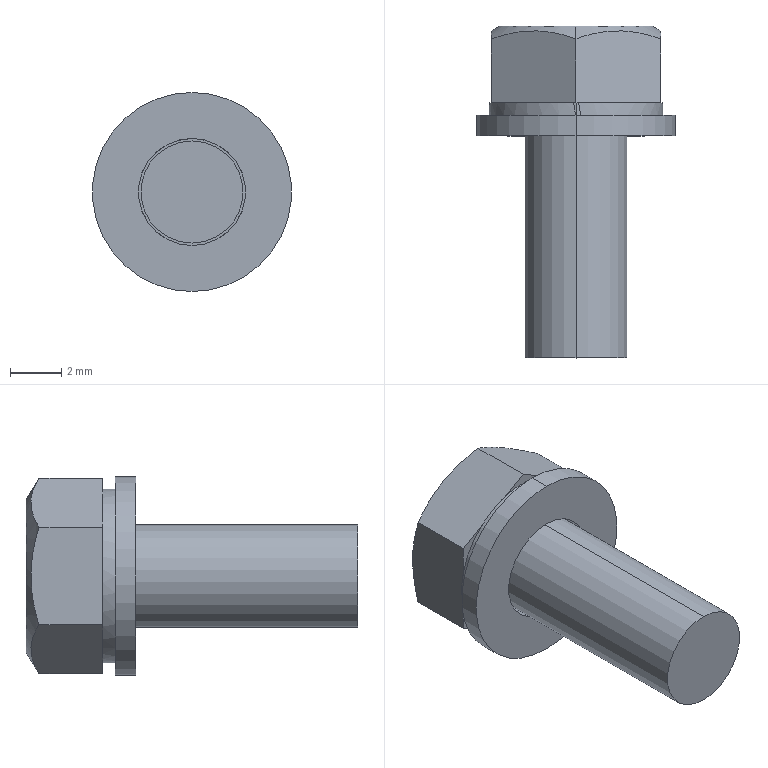Part | NX | features BREP 1 | 1 solid | 54 faces | box 7.8 x 13 x 7.8 mm | volume 254.436 mm3 | plane 38 | cylinder 10 | spline 4 | cone 2 | commonest cylinder face diameters 4 x2 4.2 x2 5.2 x2 6.8 x2 7.8 x2